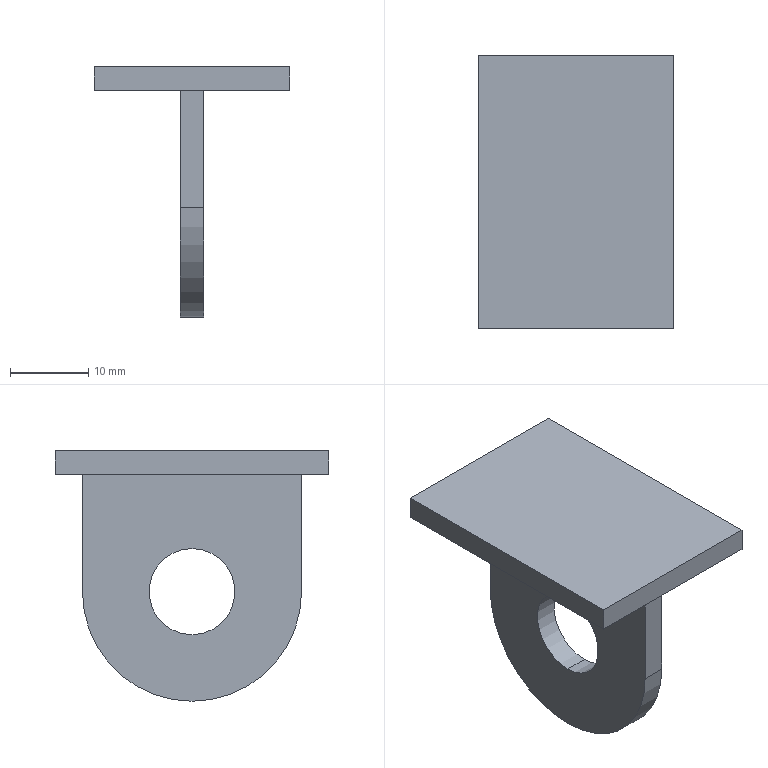Part | SolidWorks | features Extrusion 1, ICE 1 | 2 solids | 14 faces | box 25 x 35 x 32 mm | volume 4524 mm3 | plane 11 | cylinder 3 | commonest cylinder face diameters 11 x2 28 x1
STEP:
#1=CARTESIAN_POINT('',(12.5,-17.5,0.));
#2=VERTEX_POINT('',#1);
#3=CARTESIAN_POINT('',(12.5,17.5,0.));
#4=VERTEX_POINT('',#3);
#5=CARTESIAN_POINT('',(12.5,17.5,0.));
#6=DIRECTION('',(0.,1.,0.));
#7=VECTOR('',#6,1000.);
#8=LINE('',#5,#7);
#9=EDGE_CURVE('',#2,#4,#8,.T.);
#10=ORIENTED_EDGE('',*,*,#9,.T.);
#11=CARTESIAN_POINT('',(12.5,17.5,3.));
#12=VERTEX_POINT('',#11);
#13=CARTESIAN_POINT('',(12.5,17.5,3.));
#14=DIRECTION('',(0.,0.,-1.));
#15=VECTOR('',#14,1000.);
#16=LINE('',#13,#15);
#17=EDGE_CURVE('',#12,#4,#16,.T.);
#18=ORIENTED_EDGE('',*,*,#17,.F.);
#19=CARTESIAN_POINT('',(12.5,-17.5,3.));
#20=VERTEX_POINT('',#19);
#21=CARTESIAN_POINT('',(12.5,17.5,3.));
#22=DIRECTION('',(0.,1.,0.));
#23=VECTOR('',#22,1000.);
#24=LINE('',#21,#23);
#25=EDGE_CURVE('',#20,#12,#24,.T.);
#26=ORIENTED_EDGE('',*,*,#25,.F.);
#27=CARTESIAN_POINT('',(12.5,-17.5,3.));
#28=DIRECTION('',(0.,0.,-1.));
#29=VECTOR('',#28,1000.);
#30=LINE('',#27,#29);
#31=EDGE_CURVE('',#20,#2,#30,.T.);
#32=ORIENTED_EDGE('',*,*,#31,.T.);
#33=EDGE_LOOP('',(#10,#18,#26,#32));
#34=FACE_OUTER_BOUND('',#33,.T.);
#35=CARTESIAN_POINT('',(12.5,17.5,3.));
#36=DIRECTION('',(-1.,0.,0.));
#37=DIRECTION('',(0.,-1.,0.));
#38=AXIS2_PLACEMENT_3D('',#35,#36,#37);
#39=PLANE('',#38);
#40=ADVANCED_FACE('',(#34),#39,.F.);
#41=CARTESIAN_POINT('',(-12.5,17.5,0.));
#42=VERTEX_POINT('',#41);
#43=CARTESIAN_POINT('',(-12.5,17.5,0.));
#44=DIRECTION('',(-1.,0.,0.));
#45=VECTOR('',#44,1000.);
#46=LINE('',#43,#45);
#47=EDGE_CURVE('',#4,#42,#46,.T.);
#48=ORIENTED_EDGE('',*,*,#47,.T.);
#49=CARTESIAN_POINT('',(-12.5,17.5,3.));
#50=VERTEX_POINT('',#49);
#51=CARTESIAN_POINT('',(-12.5,17.5,3.));
#52=DIRECTION('',(0.,0.,-1.));
#53=VECTOR('',#52,1000.);
#54=LINE('',#51,#53);
#55=EDGE_CURVE('',#50,#42,#54,.T.);
#56=ORIENTED_EDGE('',*,*,#55,.F.);
#57=CARTESIAN_POINT('',(-12.5,17.5,3.));
#58=DIRECTION('',(-1.,0.,0.));
#59=VECTOR('',#58,1000.);
#60=LINE('',#57,#59);
#61=EDGE_CURVE('',#12,#50,#60,.T.);
#62=ORIENTED_EDGE('',*,*,#61,.F.);
#63=ORIENTED_EDGE('',*,*,#17,.T.);
#64=EDGE_LOOP('',(#48,#56,#62,#63));
#65=FACE_OUTER_BOUND('',#64,.T.);
#66=CARTESIAN_POINT('',(-12.5,17.5,3.));
#67=DIRECTION('',(0.,-1.,0.));
#68=DIRECTION('',(0.,0.,-1.));
#69=AXIS2_PLACEMENT_3D('',#66,#67,#68);
#70=PLANE('',#69);
#71=ADVANCED_FACE('',(#65),#70,.F.);
#72=CARTESIAN_POINT('',(-12.5,-17.5,0.));
#73=VERTEX_POINT('',#72);
#74=CARTESIAN_POINT('',(-12.5,17.5,0.));
#75=DIRECTION('',(0.,-1.,0.));
#76=VECTOR('',#75,1000.);
#77=LINE('',#74,#76);
#78=EDGE_CURVE('',#42,#73,#77,.T.);
#79=ORIENTED_EDGE('',*,*,#78,.T.);
#80=CARTESIAN_POINT('',(-12.5,-17.5,3.));
#81=VERTEX_POINT('',#80);
#82=CARTESIAN_POINT('',(-12.5,-17.5,3.));
#83=DIRECTION('',(0.,0.,-1.));
#84=VECTOR('',#83,1000.);
#85=LINE('',#82,#84);
#86=EDGE_CURVE('',#81,#73,#85,.T.);
#87=ORIENTED_EDGE('',*,*,#86,.F.);
#88=CARTESIAN_POINT('',(-12.5,17.5,3.));
#89=DIRECTION('',(0.,-1.,0.));
#90=VECTOR('',#89,1000.);
#91=LINE('',#88,#90);
#92=EDGE_CURVE('',#50,#81,#91,.T.);
#93=ORIENTED_EDGE('',*,*,#92,.F.);
#94=ORIENTED_EDGE('',*,*,#55,.T.);
#95=EDGE_LOOP('',(#79,#87,#93,#94));
#96=FACE_OUTER_BOUND('',#95,.T.);
#97=CARTESIAN_POINT('',(-12.5,17.5,3.));
#98=DIRECTION('',(1.,0.,0.));
#99=DIRECTION('',(0.,0.,-1.));
#100=AXIS2_PLACEMENT_3D('',#97,#98,#99);
#101=PLANE('',#100);
#102=ADVANCED_FACE('',(#96),#101,.F.);
#103=CARTESIAN_POINT('',(-12.5,-17.5,0.));
#104=DIRECTION('',(1.,0.,0.));
#105=VECTOR('',#104,1000.);
#106=LINE('',#103,#105);
#107=EDGE_CURVE('',#73,#2,#106,.T.);
#108=ORIENTED_EDGE('',*,*,#107,.T.);
#109=ORIENTED_EDGE('',*,*,#31,.F.);
#110=CARTESIAN_POINT('',(-12.5,-17.5,3.));
#111=DIRECTION('',(1.,0.,0.));
#112=VECTOR('',#111,1000.);
#113=LINE('',#110,#112);
#114=EDGE_CURVE('',#81,#20,#113,.T.);
#115=ORIENTED_EDGE('',*,*,#114,.F.);
#116=ORIENTED_EDGE('',*,*,#86,.T.);
#117=EDGE_LOOP('',(#108,#109,#115,#116));
#118=FACE_OUTER_BOUND('',#117,.T.);
#119=CARTESIAN_POINT('',(-12.5,-17.5,3.));
#120=DIRECTION('',(0.,1.,0.));
#121=DIRECTION('',(0.,0.,1.));
#122=AXIS2_PLACEMENT_3D('',#119,#120,#121);
#123=PLANE('',#122);
#124=ADVANCED_FACE('',(#118),#123,.F.);
#125=ORIENTED_EDGE('',*,*,#25,.T.);
#126=ORIENTED_EDGE('',*,*,#61,.T.);
#127=ORIENTED_EDGE('',*,*,#92,.T.);
#128=ORIENTED_EDGE('',*,*,#114,.T.);
#129=EDGE_LOOP('',(#125,#126,#127,#128));
#130=FACE_OUTER_BOUND('',#129,.T.);
#131=CARTESIAN_POINT('',(0.,0.,3.));
#132=DIRECTION('',(0.,0.,1.));
#133=DIRECTION('',(1.,0.,0.));
#134=AXIS2_PLACEMENT_3D('',#131,#132,#133);
#135=PLANE('',#134);
#136=ADVANCED_FACE('',(#130),#135,.T.);
#137=ORIENTED_EDGE('',*,*,#9,.F.);
#138=ORIENTED_EDGE('',*,*,#107,.F.);
#139=ORIENTED_EDGE('',*,*,#78,.F.);
#140=ORIENTED_EDGE('',*,*,#47,.F.);
#141=EDGE_LOOP('',(#137,#138,#139,#140));
#142=FACE_OUTER_BOUND('',#141,.T.);
#143=CARTESIAN_POINT('',(0.,0.,0.));
#144=DIRECTION('',(0.,0.,1.));
#145=DIRECTION('',(1.,0.,0.));
#146=AXIS2_PLACEMENT_3D('',#143,#144,#145);
#147=PLANE('',#146);
#148=ADVANCED_FACE('',(#142),#147,.F.);
#149=CLOSED_SHELL('',(#40,#71,#102,#124,#136,#148));
#150=MANIFOLD_SOLID_BREP('',#149);
#151=CARTESIAN_POINT('',(1.5,0.,-9.5));
#152=VERTEX_POINT('',#151);
#153=CARTESIAN_POINT('',(1.5,0.,-20.5));
#154=VERTEX_POINT('',#153);
#155=CARTESIAN_POINT('',(1.5,0.,-15.));
#156=DIRECTION('',(1.,0.,0.));
#157=DIRECTION('',(0.,0.,-1.));
#158=AXIS2_PLACEMENT_3D('',#155,#156,#157);
#159=CIRCLE('',#158,5.5);
#160=EDGE_CURVE('',#152,#154,#159,.T.);
#161=ORIENTED_EDGE('',*,*,#160,.T.);
#162=CARTESIAN_POINT('',(-1.5,0.,-20.5));
#163=VERTEX_POINT('',#162);
#164=CARTESIAN_POINT('',(1.5,0.,-20.5));
#165=DIRECTION('',(-1.,0.,0.));
#166=VECTOR('',#165,1000.);
#167=LINE('',#164,#166);
#168=EDGE_CURVE('',#154,#163,#167,.T.);
#169=ORIENTED_EDGE('',*,*,#168,.T.);
#170=CARTESIAN_POINT('',(-1.5,0.,-9.5));
#171=VERTEX_POINT('',#170);
#172=CARTESIAN_POINT('',(-1.5,0.,-15.));
#173=DIRECTION('',(1.,0.,0.));
#174=DIRECTION('',(0.,0.,-1.));
#175=AXIS2_PLACEMENT_3D('',#172,#173,#174);
#176=CIRCLE('',#175,5.5);
#177=EDGE_CURVE('',#171,#163,#176,.T.);
#178=ORIENTED_EDGE('',*,*,#177,.F.);
#179=CARTESIAN_POINT('',(1.5,0.,-9.5));
#180=DIRECTION('',(-1.,0.,0.));
#181=VECTOR('',#180,1000.);
#182=LINE('',#179,#181);
#183=EDGE_CURVE('',#152,#171,#182,.T.);
#184=ORIENTED_EDGE('',*,*,#183,.F.);
#185=EDGE_LOOP('',(#161,#169,#178,#184));
#186=FACE_OUTER_BOUND('',#185,.T.);
#187=CARTESIAN_POINT('',(1.5,0.,-15.));
#188=DIRECTION('',(-1.,0.,0.));
#189=DIRECTION('',(0.,0.,1.));
#190=AXIS2_PLACEMENT_3D('',#187,#188,#189);
#191=CYLINDRICAL_SURFACE('',#190,5.5);
#192=ADVANCED_FACE('',(#186),#191,.F.);
#193=CARTESIAN_POINT('',(1.5,14.,0.));
#194=VERTEX_POINT('',#193);
#195=CARTESIAN_POINT('',(1.5,-14.,0.));
#196=VERTEX_POINT('',#195);
#197=CARTESIAN_POINT('',(1.5,14.,0.));
#198=DIRECTION('',(0.,-1.,0.));
#199=VECTOR('',#198,1000.);
#200=LINE('',#197,#199);
#201=EDGE_CURVE('',#194,#196,#200,.T.);
#202=ORIENTED_EDGE('',*,*,#201,.T.);
#203=CARTESIAN_POINT('',(1.5,-14.,-15.));
#204=VERTEX_POINT('',#203);
#205=CARTESIAN_POINT('',(1.5,-14.,0.));
#206=DIRECTION('',(0.,0.,-1.));
#207=VECTOR('',#206,1000.);
#208=LINE('',#205,#207);
#209=EDGE_CURVE('',#196,#204,#208,.T.);
#210=ORIENTED_EDGE('',*,*,#209,.T.);
#211=CARTESIAN_POINT('',(1.5,14.,-15.));
#212=VERTEX_POINT('',#211);
#213=CARTESIAN_POINT('',(1.5,0.,-15.));
#214=DIRECTION('',(1.,0.,0.));
#215=DIRECTION('',(0.,0.,1.));
#216=AXIS2_PLACEMENT_3D('',#213,#214,#215);
#217=CIRCLE('',#216,14.);
#218=EDGE_CURVE('',#204,#212,#217,.T.);
#219=ORIENTED_EDGE('',*,*,#218,.T.);
#220=CARTESIAN_POINT('',(1.5,14.,0.));
#221=DIRECTION('',(0.,0.,1.));
#222=VECTOR('',#221,1000.);
#223=LINE('',#220,#222);
#224=EDGE_CURVE('',#212,#194,#223,.T.);
#225=ORIENTED_EDGE('',*,*,#224,.T.);
#226=EDGE_LOOP('',(#202,#210,#219,#225));
#227=FACE_OUTER_BOUND('',#226,.T.);
#228=ORIENTED_EDGE('',*,*,#160,.F.);
#229=CARTESIAN_POINT('',(1.5,0.,-15.));
#230=DIRECTION('',(1.,0.,0.));
#231=DIRECTION('',(0.,0.,-1.));
#232=AXIS2_PLACEMENT_3D('',#229,#230,#231);
#233=CIRCLE('',#232,5.5);
#234=EDGE_CURVE('',#154,#152,#233,.T.);
#235=ORIENTED_EDGE('',*,*,#234,.F.);
#236=EDGE_LOOP('',(#228,#235));
#237=FACE_BOUND('',#236,.T.);
#238=CARTESIAN_POINT('',(1.5,0.,-15.));
#239=DIRECTION('',(-1.,0.,0.));
#240=DIRECTION('',(0.,0.,1.));
#241=AXIS2_PLACEMENT_3D('',#238,#239,#240);
#242=PLANE('',#241);
#243=ADVANCED_FACE('',(#227,#237),#242,.F.);
#244=CARTESIAN_POINT('',(-1.5,14.,0.));
#245=VERTEX_POINT('',#244);
#246=CARTESIAN_POINT('',(-1.5,-14.,0.));
#247=VERTEX_POINT('',#246);
#248=CARTESIAN_POINT('',(-1.5,14.,0.));
#249=DIRECTION('',(0.,-1.,0.));
#250=VECTOR('',#249,1000.);
#251=LINE('',#248,#250);
#252=EDGE_CURVE('',#245,#247,#251,.T.);
#253=ORIENTED_EDGE('',*,*,#252,.F.);
#254=CARTESIAN_POINT('',(-1.5,14.,-15.));
#255=VERTEX_POINT('',#254);
#256=CARTESIAN_POINT('',(-1.5,14.,0.));
#257=DIRECTION('',(0.,0.,1.));
#258=VECTOR('',#257,1000.);
#259=LINE('',#256,#258);
#260=EDGE_CURVE('',#255,#245,#259,.T.);
#261=ORIENTED_EDGE('',*,*,#260,.F.);
#262=CARTESIAN_POINT('',(-1.5,-14.,-15.));
#263=VERTEX_POINT('',#262);
#264=CARTESIAN_POINT('',(-1.5,0.,-15.));
#265=DIRECTION('',(1.,0.,0.));
#266=DIRECTION('',(0.,0.,1.));
#267=AXIS2_PLACEMENT_3D('',#264,#265,#266);
#268=CIRCLE('',#267,14.);
#269=EDGE_CURVE('',#263,#255,#268,.T.);
#270=ORIENTED_EDGE('',*,*,#269,.F.);
#271=CARTESIAN_POINT('',(-1.5,-14.,0.));
#272=DIRECTION('',(0.,0.,-1.));
#273=VECTOR('',#272,1000.);
#274=LINE('',#271,#273);
#275=EDGE_CURVE('',#247,#263,#274,.T.);
#276=ORIENTED_EDGE('',*,*,#275,.F.);
#277=EDGE_LOOP('',(#253,#261,#270,#276));
#278=FACE_OUTER_BOUND('',#277,.T.);
#279=ORIENTED_EDGE('',*,*,#177,.T.);
#280=CARTESIAN_POINT('',(-1.5,0.,-15.));
#281=DIRECTION('',(1.,0.,0.));
#282=DIRECTION('',(0.,0.,-1.));
#283=AXIS2_PLACEMENT_3D('',#280,#281,#282);
#284=CIRCLE('',#283,5.5);
#285=EDGE_CURVE('',#163,#171,#284,.T.);
#286=ORIENTED_EDGE('',*,*,#285,.T.);
#287=EDGE_LOOP('',(#279,#286));
#288=FACE_BOUND('',#287,.T.);
#289=CARTESIAN_POINT('',(-1.5,0.,-15.));
#290=DIRECTION('',(-1.,0.,0.));
#291=DIRECTION('',(0.,0.,1.));
#292=AXIS2_PLACEMENT_3D('',#289,#290,#291);
#293=PLANE('',#292);
#294=ADVANCED_FACE('',(#278,#288),#293,.T.);
#295=ORIENTED_EDGE('',*,*,#252,.T.);
#296=CARTESIAN_POINT('',(1.5,-14.,0.));
#297=DIRECTION('',(-1.,0.,0.));
#298=VECTOR('',#297,1000.);
#299=LINE('',#296,#298);
#300=EDGE_CURVE('',#196,#247,#299,.T.);
#301=ORIENTED_EDGE('',*,*,#300,.F.);
#302=ORIENTED_EDGE('',*,*,#201,.F.);
#303=CARTESIAN_POINT('',(1.5,14.,0.));
#304=DIRECTION('',(-1.,0.,0.));
#305=VECTOR('',#304,1000.);
#306=LINE('',#303,#305);
#307=EDGE_CURVE('',#194,#245,#306,.T.);
#308=ORIENTED_EDGE('',*,*,#307,.T.);
#309=EDGE_LOOP('',(#295,#301,#302,#308));
#310=FACE_OUTER_BOUND('',#309,.T.);
#311=CARTESIAN_POINT('',(1.5,14.,0.));
#312=DIRECTION('',(0.,0.,-1.));
#313=DIRECTION('',(-1.,0.,0.));
#314=AXIS2_PLACEMENT_3D('',#311,#312,#313);
#315=PLANE('',#314);
#316=ADVANCED_FACE('',(#310),#315,.F.);
#317=ORIENTED_EDGE('',*,*,#275,.T.);
#318=CARTESIAN_POINT('',(1.5,-14.,-15.));
#319=DIRECTION('',(-1.,0.,0.));
#320=VECTOR('',#319,1000.);
#321=LINE('',#318,#320);
#322=EDGE_CURVE('',#204,#263,#321,.T.);
#323=ORIENTED_EDGE('',*,*,#322,.F.);
#324=ORIENTED_EDGE('',*,*,#209,.F.);
#325=ORIENTED_EDGE('',*,*,#300,.T.);
#326=EDGE_LOOP('',(#317,#323,#324,#325));
#327=FACE_OUTER_BOUND('',#326,.T.);
#328=CARTESIAN_POINT('',(1.5,-14.,0.));
#329=DIRECTION('',(0.,1.,0.));
#330=DIRECTION('',(0.,0.,1.));
#331=AXIS2_PLACEMENT_3D('',#328,#329,#330);
#332=PLANE('',#331);
#333=ADVANCED_FACE('',(#327),#332,.F.);
#334=ORIENTED_EDGE('',*,*,#269,.T.);
#335=CARTESIAN_POINT('',(1.5,14.,-15.));
#336=DIRECTION('',(-1.,0.,0.));
#337=VECTOR('',#336,1000.);
#338=LINE('',#335,#337);
#339=EDGE_CURVE('',#212,#255,#338,.T.);
#340=ORIENTED_EDGE('',*,*,#339,.F.);
#341=ORIENTED_EDGE('',*,*,#218,.F.);
#342=ORIENTED_EDGE('',*,*,#322,.T.);
#343=EDGE_LOOP('',(#334,#340,#341,#342));
#344=FACE_OUTER_BOUND('',#343,.T.);
#345=CARTESIAN_POINT('',(1.5,0.,-15.));
#346=DIRECTION('',(-1.,0.,0.));
#347=DIRECTION('',(0.,0.,1.));
#348=AXIS2_PLACEMENT_3D('',#345,#346,#347);
#349=CYLINDRICAL_SURFACE('',#348,14.);
#350=ADVANCED_FACE('',(#344),#349,.T.);
#351=ORIENTED_EDGE('',*,*,#260,.T.);
#352=ORIENTED_EDGE('',*,*,#307,.F.);
#353=ORIENTED_EDGE('',*,*,#224,.F.);
#354=ORIENTED_EDGE('',*,*,#339,.T.);
#355=EDGE_LOOP('',(#351,#352,#353,#354));
#356=FACE_OUTER_BOUND('',#355,.T.);
#357=CARTESIAN_POINT('',(1.5,14.,0.));
#358=DIRECTION('',(0.,-1.,0.));
#359=DIRECTION('',(0.,0.,-1.));
#360=AXIS2_PLACEMENT_3D('',#357,#358,#359);
#361=PLANE('',#360);
#362=ADVANCED_FACE('',(#356),#361,.F.);
#363=ORIENTED_EDGE('',*,*,#168,.F.);
#364=ORIENTED_EDGE('',*,*,#234,.T.);
#365=ORIENTED_EDGE('',*,*,#183,.T.);
#366=ORIENTED_EDGE('',*,*,#285,.F.);
#367=EDGE_LOOP('',(#363,#364,#365,#366));
#368=FACE_OUTER_BOUND('',#367,.T.);
#369=CARTESIAN_POINT('',(1.5,0.,-15.));
#370=DIRECTION('',(-1.,0.,0.));
#371=DIRECTION('',(0.,0.,1.));
#372=AXIS2_PLACEMENT_3D('',#369,#370,#371);
#373=CYLINDRICAL_SURFACE('',#372,5.5);
#374=ADVANCED_FACE('',(#368),#373,.F.);
#375=CLOSED_SHELL('',(#192,#243,#294,#316,#333,#350,#362,#374));
#376=MANIFOLD_SOLID_BREP('',#375);
#377=CARTESIAN_POINT('',(0.,0.,0.));
#378=DIRECTION('',(0.,0.,1.));
#379=DIRECTION('',(1.,0.,0.));
#380=AXIS2_PLACEMENT_3D('',#377,#378,#379);
#381=(LENGTH_UNIT()NAMED_UNIT(*)SI_UNIT(.MILLI.,.METRE.));
#382=UNCERTAINTY_MEASURE_WITH_UNIT(LENGTH_MEASURE(0.00001),#381,'','');
#383=(NAMED_UNIT(*)PLANE_ANGLE_UNIT()SI_UNIT($,.RADIAN.));
#384=(NAMED_UNIT(*)SI_UNIT($,.STERADIAN.)SOLID_ANGLE_UNIT());
#385=(GEOMETRIC_REPRESENTATION_CONTEXT(3)GLOBAL_UNCERTAINTY_ASSIGNED_CONTEXT((#382))GLOBAL_UNIT_ASSIGNED_CONTEXT((#381,#383,#384))REPRESENTATION_CONTEXT('',''));
#386=ADVANCED_BREP_SHAPE_REPRESENTATION('',(#150,#376,#380),#385);